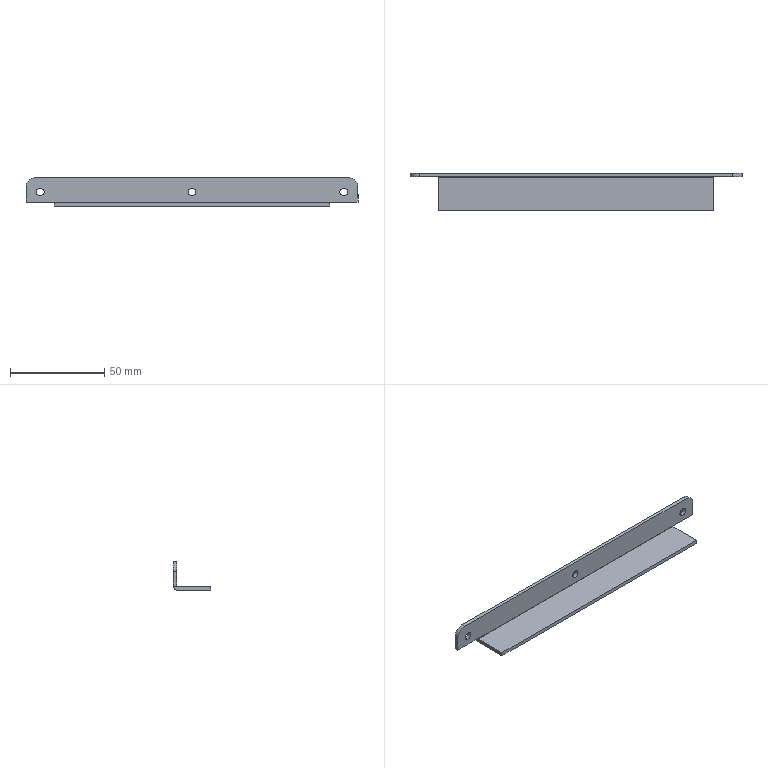Part | SolidWorks | features BaseBody 1 | 1 solid | 22 faces | box 176 x 20 x 15 mm | volume 10168 mm3 | plane 12 | cylinder 10 | commonest cylinder face diameters 4.2 x7 10 x2 0.2 x1
STEP:
#1=CARTESIAN_POINT('',(80.5,8.,3.4));
#2=VERTEX_POINT('',#1);
#3=CARTESIAN_POINT('',(80.5,8.,7.6));
#4=VERTEX_POINT('',#3);
#5=CARTESIAN_POINT('',(80.5,8.,5.5));
#6=DIRECTION('',(0.,1.,0.));
#7=DIRECTION('',(0.,0.,1.));
#8=AXIS2_PLACEMENT_3D('',#5,#6,#7);
#9=CIRCLE('',#8,2.1);
#10=EDGE_CURVE('',#2,#4,#9,.T.);
#11=ORIENTED_EDGE('',*,*,#10,.F.);
#12=CARTESIAN_POINT('',(80.5,10.,3.4));
#13=VERTEX_POINT('',#12);
#14=CARTESIAN_POINT('',(80.5,10.,3.4));
#15=DIRECTION('',(0.,1.,0.));
#16=VECTOR('',#15,1000.);
#17=LINE('',#14,#16);
#18=EDGE_CURVE('',#2,#13,#17,.T.);
#19=ORIENTED_EDGE('',*,*,#18,.T.);
#20=CARTESIAN_POINT('',(80.5,10.,7.6));
#21=VERTEX_POINT('',#20);
#22=CARTESIAN_POINT('',(80.5,10.,5.5));
#23=DIRECTION('',(0.,1.,0.));
#24=DIRECTION('',(0.,0.,1.));
#25=AXIS2_PLACEMENT_3D('',#22,#23,#24);
#26=CIRCLE('',#25,2.1);
#27=EDGE_CURVE('',#13,#21,#26,.T.);
#28=ORIENTED_EDGE('',*,*,#27,.T.);
#29=CARTESIAN_POINT('',(80.5,10.,7.6));
#30=DIRECTION('',(0.,1.,0.));
#31=VECTOR('',#30,1000.);
#32=LINE('',#29,#31);
#33=EDGE_CURVE('',#4,#21,#32,.T.);
#34=ORIENTED_EDGE('',*,*,#33,.F.);
#35=EDGE_LOOP('',(#11,#19,#28,#34));
#36=FACE_OUTER_BOUND('',#35,.T.);
#37=CARTESIAN_POINT('',(80.5,10.,5.5));
#38=DIRECTION('',(0.,1.,0.));
#39=DIRECTION('',(0.,0.,1.));
#40=AXIS2_PLACEMENT_3D('',#37,#38,#39);
#41=CYLINDRICAL_SURFACE('',#40,2.1);
#42=ADVANCED_FACE('',(#36),#41,.F.);
#43=CARTESIAN_POINT('',(0.,8.,3.4));
#44=VERTEX_POINT('',#43);
#45=CARTESIAN_POINT('',(0.,8.,7.6));
#46=VERTEX_POINT('',#45);
#47=CARTESIAN_POINT('',(0.,8.,5.5));
#48=DIRECTION('',(0.,1.,0.));
#49=DIRECTION('',(0.,0.,1.));
#50=AXIS2_PLACEMENT_3D('',#47,#48,#49);
#51=CIRCLE('',#50,2.1);
#52=EDGE_CURVE('',#44,#46,#51,.T.);
#53=ORIENTED_EDGE('',*,*,#52,.F.);
#54=CARTESIAN_POINT('',(0.,10.,3.4));
#55=VERTEX_POINT('',#54);
#56=CARTESIAN_POINT('',(0.,10.,3.4));
#57=DIRECTION('',(0.,1.,0.));
#58=VECTOR('',#57,1000.);
#59=LINE('',#56,#58);
#60=EDGE_CURVE('',#44,#55,#59,.T.);
#61=ORIENTED_EDGE('',*,*,#60,.T.);
#62=CARTESIAN_POINT('',(0.,10.,7.6));
#63=VERTEX_POINT('',#62);
#64=CARTESIAN_POINT('',(0.,10.,5.5));
#65=DIRECTION('',(0.,1.,0.));
#66=DIRECTION('',(0.,0.,1.));
#67=AXIS2_PLACEMENT_3D('',#64,#65,#66);
#68=CIRCLE('',#67,2.1);
#69=EDGE_CURVE('',#55,#63,#68,.T.);
#70=ORIENTED_EDGE('',*,*,#69,.T.);
#71=CARTESIAN_POINT('',(0.,10.,7.6));
#72=DIRECTION('',(0.,1.,0.));
#73=VECTOR('',#72,1000.);
#74=LINE('',#71,#73);
#75=EDGE_CURVE('',#46,#63,#74,.T.);
#76=ORIENTED_EDGE('',*,*,#75,.F.);
#77=EDGE_LOOP('',(#53,#61,#70,#76));
#78=FACE_OUTER_BOUND('',#77,.T.);
#79=CARTESIAN_POINT('',(0.,10.,5.5));
#80=DIRECTION('',(0.,1.,0.));
#81=DIRECTION('',(0.,0.,1.));
#82=AXIS2_PLACEMENT_3D('',#79,#80,#81);
#83=CYLINDRICAL_SURFACE('',#82,2.1);
#84=ADVANCED_FACE('',(#78),#83,.F.);
#85=CARTESIAN_POINT('',(-80.5,8.,3.4));
#86=VERTEX_POINT('',#85);
#87=CARTESIAN_POINT('',(-80.5,8.,7.6));
#88=VERTEX_POINT('',#87);
#89=CARTESIAN_POINT('',(-80.5,8.,5.5));
#90=DIRECTION('',(0.,1.,0.));
#91=DIRECTION('',(0.,0.,1.));
#92=AXIS2_PLACEMENT_3D('',#89,#90,#91);
#93=CIRCLE('',#92,2.1);
#94=EDGE_CURVE('',#86,#88,#93,.T.);
#95=ORIENTED_EDGE('',*,*,#94,.F.);
#96=CARTESIAN_POINT('',(-80.5,10.,3.4));
#97=VERTEX_POINT('',#96);
#98=CARTESIAN_POINT('',(-80.5,10.,3.4));
#99=DIRECTION('',(0.,1.,0.));
#100=VECTOR('',#99,1000.);
#101=LINE('',#98,#100);
#102=EDGE_CURVE('',#86,#97,#101,.T.);
#103=ORIENTED_EDGE('',*,*,#102,.T.);
#104=CARTESIAN_POINT('',(-80.5,10.,7.6));
#105=VERTEX_POINT('',#104);
#106=CARTESIAN_POINT('',(-80.5,10.,5.5));
#107=DIRECTION('',(0.,1.,0.));
#108=DIRECTION('',(0.,0.,1.));
#109=AXIS2_PLACEMENT_3D('',#106,#107,#108);
#110=CIRCLE('',#109,2.1);
#111=EDGE_CURVE('',#97,#105,#110,.T.);
#112=ORIENTED_EDGE('',*,*,#111,.T.);
#113=CARTESIAN_POINT('',(-80.5,10.,7.6));
#114=DIRECTION('',(0.,1.,0.));
#115=VECTOR('',#114,1000.);
#116=LINE('',#113,#115);
#117=EDGE_CURVE('',#88,#105,#116,.T.);
#118=ORIENTED_EDGE('',*,*,#117,.F.);
#119=EDGE_LOOP('',(#95,#103,#112,#118));
#120=FACE_OUTER_BOUND('',#119,.T.);
#121=CARTESIAN_POINT('',(-80.5,10.,5.5));
#122=DIRECTION('',(0.,1.,0.));
#123=DIRECTION('',(0.,0.,1.));
#124=AXIS2_PLACEMENT_3D('',#121,#122,#123);
#125=CYLINDRICAL_SURFACE('',#124,2.1);
#126=ADVANCED_FACE('',(#120),#125,.F.);
#127=CARTESIAN_POINT('',(73.,-10.,-2.));
#128=VERTEX_POINT('',#127);
#129=CARTESIAN_POINT('',(73.,7.9,-2.));
#130=VERTEX_POINT('',#129);
#131=CARTESIAN_POINT('',(73.,0.,-2.));
#132=DIRECTION('',(0.,1.,0.));
#133=VECTOR('',#132,1000.);
#134=LINE('',#131,#133);
#135=EDGE_CURVE('',#128,#130,#134,.T.);
#136=ORIENTED_EDGE('',*,*,#135,.F.);
#137=CARTESIAN_POINT('',(-73.,-10.,-2.));
#138=VERTEX_POINT('',#137);
#139=CARTESIAN_POINT('',(0.,-10.,-2.));
#140=DIRECTION('',(1.,0.,0.));
#141=VECTOR('',#140,1000.);
#142=LINE('',#139,#141);
#143=EDGE_CURVE('',#138,#128,#142,.T.);
#144=ORIENTED_EDGE('',*,*,#143,.F.);
#145=CARTESIAN_POINT('',(-73.,7.9,-2.));
#146=VERTEX_POINT('',#145);
#147=CARTESIAN_POINT('',(-73.,0.,-2.));
#148=DIRECTION('',(0.,-1.,0.));
#149=VECTOR('',#148,1000.);
#150=LINE('',#147,#149);
#151=EDGE_CURVE('',#146,#138,#150,.T.);
#152=ORIENTED_EDGE('',*,*,#151,.F.);
#153=CARTESIAN_POINT('',(0.,7.9,-2.));
#154=DIRECTION('',(-1.,0.,0.));
#155=VECTOR('',#154,1000.);
#156=LINE('',#153,#155);
#157=EDGE_CURVE('',#130,#146,#156,.T.);
#158=ORIENTED_EDGE('',*,*,#157,.F.);
#159=EDGE_LOOP('',(#136,#144,#152,#158));
#160=FACE_OUTER_BOUND('',#159,.T.);
#161=CARTESIAN_POINT('',(0.,0.,-2.));
#162=DIRECTION('',(0.,0.,1.));
#163=DIRECTION('',(1.,0.,0.));
#164=AXIS2_PLACEMENT_3D('',#161,#162,#163);
#165=PLANE('',#164);
#166=ADVANCED_FACE('',(#160),#165,.F.);
#167=CARTESIAN_POINT('',(-73.,10.,0.1));
#168=VERTEX_POINT('',#167);
#169=CARTESIAN_POINT('',(73.,10.,0.1));
#170=VERTEX_POINT('',#169);
#171=CARTESIAN_POINT('',(-73.,10.,0.1));
#172=DIRECTION('',(1.,0.,0.));
#173=VECTOR('',#172,1000.);
#174=LINE('',#171,#173);
#175=EDGE_CURVE('',#168,#170,#174,.T.);
#176=ORIENTED_EDGE('',*,*,#175,.T.);
#177=CARTESIAN_POINT('',(73.,7.9,0.1));
#178=DIRECTION('',(-1.,0.,0.));
#179=DIRECTION('',(0.,0.,1.));
#180=AXIS2_PLACEMENT_3D('',#177,#178,#179);
#181=CIRCLE('',#180,2.1);
#182=EDGE_CURVE('',#170,#130,#181,.T.);
#183=ORIENTED_EDGE('',*,*,#182,.T.);
#184=ORIENTED_EDGE('',*,*,#157,.T.);
#185=CARTESIAN_POINT('',(-73.,7.9,0.1));
#186=DIRECTION('',(1.,0.,0.));
#187=DIRECTION('',(0.,0.,1.));
#188=AXIS2_PLACEMENT_3D('',#185,#186,#187);
#189=CIRCLE('',#188,2.1);
#190=EDGE_CURVE('',#146,#168,#189,.T.);
#191=ORIENTED_EDGE('',*,*,#190,.T.);
#192=EDGE_LOOP('',(#176,#183,#184,#191));
#193=FACE_OUTER_BOUND('',#192,.T.);
#194=CARTESIAN_POINT('',(-73.,7.9,0.1));
#195=DIRECTION('',(-1.,0.,0.));
#196=DIRECTION('',(0.,0.,1.));
#197=AXIS2_PLACEMENT_3D('',#194,#195,#196);
#198=CYLINDRICAL_SURFACE('',#197,2.1);
#199=ADVANCED_FACE('',(#193),#198,.T.);
#200=CARTESIAN_POINT('',(73.,-10.,0.));
#201=VERTEX_POINT('',#200);
#202=CARTESIAN_POINT('',(73.,-10.,-2.));
#203=DIRECTION('',(0.,0.,-1.));
#204=VECTOR('',#203,1000.);
#205=LINE('',#202,#204);
#206=EDGE_CURVE('',#201,#128,#205,.T.);
#207=ORIENTED_EDGE('',*,*,#206,.T.);
#208=ORIENTED_EDGE('',*,*,#135,.T.);
#209=ORIENTED_EDGE('',*,*,#182,.F.);
#210=CARTESIAN_POINT('',(73.,8.,0.1));
#211=VERTEX_POINT('',#210);
#212=CARTESIAN_POINT('',(73.,7.9,0.1));
#213=DIRECTION('',(0.,-1.,0.));
#214=VECTOR('',#213,1000.);
#215=LINE('',#212,#214);
#216=EDGE_CURVE('',#170,#211,#215,.T.);
#217=ORIENTED_EDGE('',*,*,#216,.T.);
#218=CARTESIAN_POINT('',(73.,7.9,0.));
#219=VERTEX_POINT('',#218);
#220=CARTESIAN_POINT('',(73.,7.9,0.1));
#221=DIRECTION('',(-1.,0.,0.));
#222=DIRECTION('',(0.,0.,1.));
#223=AXIS2_PLACEMENT_3D('',#220,#221,#222);
#224=CIRCLE('',#223,0.1);
#225=EDGE_CURVE('',#211,#219,#224,.T.);
#226=ORIENTED_EDGE('',*,*,#225,.T.);
#227=CARTESIAN_POINT('',(73.,10.,0.));
#228=DIRECTION('',(0.,-1.,0.));
#229=VECTOR('',#228,1000.);
#230=LINE('',#227,#229);
#231=EDGE_CURVE('',#219,#201,#230,.T.);
#232=ORIENTED_EDGE('',*,*,#231,.T.);
#233=EDGE_LOOP('',(#207,#208,#209,#217,#226,#232));
#234=FACE_OUTER_BOUND('',#233,.T.);
#235=CARTESIAN_POINT('',(73.,10.,-2.));
#236=DIRECTION('',(1.,0.,0.));
#237=DIRECTION('',(0.,0.,-1.));
#238=AXIS2_PLACEMENT_3D('',#235,#236,#237);
#239=PLANE('',#238);
#240=ADVANCED_FACE('',(#234),#239,.T.);
#241=ORIENTED_EDGE('',*,*,#143,.T.);
#242=ORIENTED_EDGE('',*,*,#206,.F.);
#243=CARTESIAN_POINT('',(-73.,-10.,0.));
#244=VERTEX_POINT('',#243);
#245=CARTESIAN_POINT('',(-73.,-10.,0.));
#246=DIRECTION('',(-1.,0.,0.));
#247=VECTOR('',#246,1000.);
#248=LINE('',#245,#247);
#249=EDGE_CURVE('',#201,#244,#248,.T.);
#250=ORIENTED_EDGE('',*,*,#249,.T.);
#251=CARTESIAN_POINT('',(-73.,-10.,-2.));
#252=DIRECTION('',(0.,0.,-1.));
#253=VECTOR('',#252,1000.);
#254=LINE('',#251,#253);
#255=EDGE_CURVE('',#244,#138,#254,.T.);
#256=ORIENTED_EDGE('',*,*,#255,.T.);
#257=EDGE_LOOP('',(#241,#242,#250,#256));
#258=FACE_OUTER_BOUND('',#257,.T.);
#259=CARTESIAN_POINT('',(-73.,-10.,-2.));
#260=DIRECTION('',(0.,-1.,0.));
#261=DIRECTION('',(0.,0.,-1.));
#262=AXIS2_PLACEMENT_3D('',#259,#260,#261);
#263=PLANE('',#262);
#264=ADVANCED_FACE('',(#258),#263,.T.);
#265=ORIENTED_EDGE('',*,*,#151,.T.);
#266=ORIENTED_EDGE('',*,*,#255,.F.);
#267=CARTESIAN_POINT('',(-73.,7.9,0.));
#268=VERTEX_POINT('',#267);
#269=CARTESIAN_POINT('',(-73.,10.,0.));
#270=DIRECTION('',(0.,1.,0.));
#271=VECTOR('',#270,1000.);
#272=LINE('',#269,#271);
#273=EDGE_CURVE('',#244,#268,#272,.T.);
#274=ORIENTED_EDGE('',*,*,#273,.T.);
#275=CARTESIAN_POINT('',(-73.,8.,0.1));
#276=VERTEX_POINT('',#275);
#277=CARTESIAN_POINT('',(-73.,7.9,0.1));
#278=DIRECTION('',(1.,0.,0.));
#279=DIRECTION('',(0.,0.,1.));
#280=AXIS2_PLACEMENT_3D('',#277,#278,#279);
#281=CIRCLE('',#280,0.1);
#282=EDGE_CURVE('',#268,#276,#281,.T.);
#283=ORIENTED_EDGE('',*,*,#282,.T.);
#284=CARTESIAN_POINT('',(-73.,7.9,0.1));
#285=DIRECTION('',(0.,-1.,0.));
#286=VECTOR('',#285,1000.);
#287=LINE('',#284,#286);
#288=EDGE_CURVE('',#168,#276,#287,.T.);
#289=ORIENTED_EDGE('',*,*,#288,.F.);
#290=ORIENTED_EDGE('',*,*,#190,.F.);
#291=EDGE_LOOP('',(#265,#266,#274,#283,#289,#290));
#292=FACE_OUTER_BOUND('',#291,.T.);
#293=CARTESIAN_POINT('',(-73.,10.,-2.));
#294=DIRECTION('',(-1.,0.,0.));
#295=DIRECTION('',(0.,0.,1.));
#296=AXIS2_PLACEMENT_3D('',#293,#294,#295);
#297=PLANE('',#296);
#298=ADVANCED_FACE('',(#292),#297,.T.);
#299=CARTESIAN_POINT('',(88.,10.,8.));
#300=VERTEX_POINT('',#299);
#301=CARTESIAN_POINT('',(83.,10.,13.));
#302=VERTEX_POINT('',#301);
#303=CARTESIAN_POINT('',(83.,10.,8.));
#304=DIRECTION('',(0.,-1.,0.));
#305=DIRECTION('',(0.,0.,1.));
#306=AXIS2_PLACEMENT_3D('',#303,#304,#305);
#307=CIRCLE('',#306,5.);
#308=EDGE_CURVE('',#300,#302,#307,.T.);
#309=ORIENTED_EDGE('',*,*,#308,.F.);
#310=CARTESIAN_POINT('',(88.,10.,0.1));
#311=VERTEX_POINT('',#310);
#312=CARTESIAN_POINT('',(88.,10.,0.));
#313=DIRECTION('',(0.,0.,1.));
#314=VECTOR('',#313,1000.);
#315=LINE('',#312,#314);
#316=EDGE_CURVE('',#311,#300,#315,.T.);
#317=ORIENTED_EDGE('',*,*,#316,.F.);
#318=CARTESIAN_POINT('',(0.,10.,0.1));
#319=DIRECTION('',(1.,0.,0.));
#320=VECTOR('',#319,1000.);
#321=LINE('',#318,#320);
#322=EDGE_CURVE('',#170,#311,#321,.T.);
#323=ORIENTED_EDGE('',*,*,#322,.F.);
#324=ORIENTED_EDGE('',*,*,#175,.F.);
#325=CARTESIAN_POINT('',(-88.,10.,0.1));
#326=VERTEX_POINT('',#325);
#327=CARTESIAN_POINT('',(0.,10.,0.1));
#328=DIRECTION('',(1.,0.,0.));
#329=VECTOR('',#328,1000.);
#330=LINE('',#327,#329);
#331=EDGE_CURVE('',#326,#168,#330,.T.);
#332=ORIENTED_EDGE('',*,*,#331,.F.);
#333=CARTESIAN_POINT('',(-88.,10.,8.));
#334=VERTEX_POINT('',#333);
#335=CARTESIAN_POINT('',(-88.,10.,0.));
#336=DIRECTION('',(0.,0.,-1.));
#337=VECTOR('',#336,1000.);
#338=LINE('',#335,#337);
#339=EDGE_CURVE('',#334,#326,#338,.T.);
#340=ORIENTED_EDGE('',*,*,#339,.F.);
#341=CARTESIAN_POINT('',(-83.,10.,13.));
#342=VERTEX_POINT('',#341);
#343=CARTESIAN_POINT('',(-83.,10.,8.));
#344=DIRECTION('',(0.,-1.,0.));
#345=DIRECTION('',(0.,0.,-1.));
#346=AXIS2_PLACEMENT_3D('',#343,#344,#345);
#347=CIRCLE('',#346,5.);
#348=EDGE_CURVE('',#342,#334,#347,.T.);
#349=ORIENTED_EDGE('',*,*,#348,.F.);
#350=CARTESIAN_POINT('',(0.,10.,13.));
#351=DIRECTION('',(-1.,0.,0.));
#352=VECTOR('',#351,1000.);
#353=LINE('',#350,#352);
#354=EDGE_CURVE('',#302,#342,#353,.T.);
#355=ORIENTED_EDGE('',*,*,#354,.F.);
#356=EDGE_LOOP('',(#309,#317,#323,#324,#332,#340,#349,#355));
#357=FACE_OUTER_BOUND('',#356,.T.);
#358=CARTESIAN_POINT('',(80.5,10.,5.5));
#359=DIRECTION('',(0.,1.,0.));
#360=DIRECTION('',(0.,0.,1.));
#361=AXIS2_PLACEMENT_3D('',#358,#359,#360);
#362=CIRCLE('',#361,2.1);
#363=EDGE_CURVE('',#21,#13,#362,.T.);
#364=ORIENTED_EDGE('',*,*,#363,.F.);
#365=ORIENTED_EDGE('',*,*,#27,.F.);
#366=EDGE_LOOP('',(#364,#365));
#367=FACE_BOUND('',#366,.T.);
#368=CARTESIAN_POINT('',(0.,10.,5.5));
#369=DIRECTION('',(0.,1.,0.));
#370=DIRECTION('',(0.,0.,1.));
#371=AXIS2_PLACEMENT_3D('',#368,#369,#370);
#372=CIRCLE('',#371,2.1);
#373=EDGE_CURVE('',#63,#55,#372,.T.);
#374=ORIENTED_EDGE('',*,*,#373,.F.);
#375=ORIENTED_EDGE('',*,*,#69,.F.);
#376=EDGE_LOOP('',(#374,#375));
#377=FACE_BOUND('',#376,.T.);
#378=CARTESIAN_POINT('',(-80.5,10.,5.5));
#379=DIRECTION('',(0.,1.,0.));
#380=DIRECTION('',(0.,0.,1.));
#381=AXIS2_PLACEMENT_3D('',#378,#379,#380);
#382=CIRCLE('',#381,2.1);
#383=EDGE_CURVE('',#105,#97,#382,.T.);
#384=ORIENTED_EDGE('',*,*,#383,.F.);
#385=ORIENTED_EDGE('',*,*,#111,.F.);
#386=EDGE_LOOP('',(#384,#385));
#387=FACE_BOUND('',#386,.T.);
#388=CARTESIAN_POINT('',(0.,10.,0.));
#389=DIRECTION('',(0.,-1.,0.));
#390=DIRECTION('',(0.,0.,-1.));
#391=AXIS2_PLACEMENT_3D('',#388,#389,#390);
#392=PLANE('',#391);
#393=ADVANCED_FACE('',(#357,#367,#377,#387),#392,.F.);
#394=ORIENTED_EDGE('',*,*,#273,.F.);
#395=ORIENTED_EDGE('',*,*,#249,.F.);
#396=ORIENTED_EDGE('',*,*,#231,.F.);
#397=CARTESIAN_POINT('',(0.,7.9,0.));
#398=DIRECTION('',(-1.,0.,0.));
#399=VECTOR('',#398,1000.);
#400=LINE('',#397,#399);
#401=EDGE_CURVE('',#219,#268,#400,.T.);
#402=ORIENTED_EDGE('',*,*,#401,.T.);
#403=EDGE_LOOP('',(#394,#395,#396,#402));
#404=FACE_OUTER_BOUND('',#403,.T.);
#405=CARTESIAN_POINT('',(0.,0.,0.));
#406=DIRECTION('',(0.,0.,1.));
#407=DIRECTION('',(1.,0.,0.));
#408=AXIS2_PLACEMENT_3D('',#405,#406,#407);
#409=PLANE('',#408);
#410=ADVANCED_FACE('',(#404),#409,.T.);
#411=ORIENTED_EDGE('',*,*,#322,.T.);
#412=CARTESIAN_POINT('',(88.,8.,0.1));
#413=VERTEX_POINT('',#412);
#414=CARTESIAN_POINT('',(88.,8.,0.1));
#415=DIRECTION('',(0.,1.,0.));
#416=VECTOR('',#415,1000.);
#417=LINE('',#414,#416);
#418=EDGE_CURVE('',#413,#311,#417,.T.);
#419=ORIENTED_EDGE('',*,*,#418,.F.);
#420=CARTESIAN_POINT('',(88.,8.,0.1));
#421=DIRECTION('',(1.,0.,0.));
#422=VECTOR('',#421,1000.);
#423=LINE('',#420,#422);
#424=EDGE_CURVE('',#211,#413,#423,.T.);
#425=ORIENTED_EDGE('',*,*,#424,.F.);
#426=ORIENTED_EDGE('',*,*,#216,.F.);
#427=EDGE_LOOP('',(#411,#419,#425,#426));
#428=FACE_OUTER_BOUND('',#427,.T.);
#429=CARTESIAN_POINT('',(88.,8.,0.1));
#430=DIRECTION('',(0.,0.,1.));
#431=DIRECTION('',(0.,-1.,0.));
#432=AXIS2_PLACEMENT_3D('',#429,#430,#431);
#433=PLANE('',#432);
#434=ADVANCED_FACE('',(#428),#433,.F.);
#435=CARTESIAN_POINT('',(83.,8.,13.));
#436=VERTEX_POINT('',#435);
#437=CARTESIAN_POINT('',(83.,10.,13.));
#438=DIRECTION('',(0.,-1.,0.));
#439=VECTOR('',#438,1000.);
#440=LINE('',#437,#439);
#441=EDGE_CURVE('',#302,#436,#440,.T.);
#442=ORIENTED_EDGE('',*,*,#441,.F.);
#443=ORIENTED_EDGE('',*,*,#354,.T.);
#444=CARTESIAN_POINT('',(-83.,8.,13.));
#445=VERTEX_POINT('',#444);
#446=CARTESIAN_POINT('',(-83.,10.,13.));
#447=DIRECTION('',(0.,1.,0.));
#448=VECTOR('',#447,1000.);
#449=LINE('',#446,#448);
#450=EDGE_CURVE('',#445,#342,#449,.T.);
#451=ORIENTED_EDGE('',*,*,#450,.F.);
#452=CARTESIAN_POINT('',(73.,8.,13.));
#453=DIRECTION('',(-1.,0.,0.));
#454=VECTOR('',#453,1000.);
#455=LINE('',#452,#454);
#456=EDGE_CURVE('',#436,#445,#455,.T.);
#457=ORIENTED_EDGE('',*,*,#456,.F.);
#458=EDGE_LOOP('',(#442,#443,#451,#457));
#459=FACE_OUTER_BOUND('',#458,.T.);
#460=CARTESIAN_POINT('',(73.,10.,13.));
#461=DIRECTION('',(0.,0.,-1.));
#462=DIRECTION('',(0.,1.,0.));
#463=AXIS2_PLACEMENT_3D('',#460,#461,#462);
#464=PLANE('',#463);
#465=ADVANCED_FACE('',(#459),#464,.F.);
#466=CARTESIAN_POINT('',(88.,8.,8.));
#467=VERTEX_POINT('',#466);
#468=CARTESIAN_POINT('',(83.,8.,8.));
#469=DIRECTION('',(0.,1.,0.));
#470=DIRECTION('',(0.,0.,1.));
#471=AXIS2_PLACEMENT_3D('',#468,#469,#470);
#472=CIRCLE('',#471,5.);
#473=EDGE_CURVE('',#436,#467,#472,.T.);
#474=ORIENTED_EDGE('',*,*,#473,.T.);
#475=CARTESIAN_POINT('',(88.,0.,8.));
#476=DIRECTION('',(0.,1.,0.));
#477=VECTOR('',#476,1000.);
#478=LINE('',#475,#477);
#479=EDGE_CURVE('',#467,#300,#478,.T.);
#480=ORIENTED_EDGE('',*,*,#479,.T.);
#481=ORIENTED_EDGE('',*,*,#308,.T.);
#482=ORIENTED_EDGE('',*,*,#441,.T.);
#483=EDGE_LOOP('',(#474,#480,#481,#482));
#484=FACE_OUTER_BOUND('',#483,.T.);
#485=CARTESIAN_POINT('',(83.,0.,8.));
#486=DIRECTION('',(0.,1.,0.));
#487=DIRECTION('',(0.,0.,1.));
#488=AXIS2_PLACEMENT_3D('',#485,#486,#487);
#489=CYLINDRICAL_SURFACE('',#488,5.);
#490=ADVANCED_FACE('',(#484),#489,.T.);
#491=CARTESIAN_POINT('',(88.,8.,0.));
#492=DIRECTION('',(0.,0.,-1.));
#493=VECTOR('',#492,1000.);
#494=LINE('',#491,#493);
#495=EDGE_CURVE('',#467,#413,#494,.T.);
#496=ORIENTED_EDGE('',*,*,#495,.T.);
#497=ORIENTED_EDGE('',*,*,#418,.T.);
#498=ORIENTED_EDGE('',*,*,#316,.T.);
#499=ORIENTED_EDGE('',*,*,#479,.F.);
#500=EDGE_LOOP('',(#496,#497,#498,#499));
#501=FACE_OUTER_BOUND('',#500,.T.);
#502=CARTESIAN_POINT('',(88.,0.,0.));
#503=DIRECTION('',(1.,0.,0.));
#504=DIRECTION('',(0.,0.,-1.));
#505=AXIS2_PLACEMENT_3D('',#502,#503,#504);
#506=PLANE('',#505);
#507=ADVANCED_FACE('',(#501),#506,.T.);
#508=CARTESIAN_POINT('',(-88.,8.,0.1));
#509=VERTEX_POINT('',#508);
#510=CARTESIAN_POINT('',(-88.,8.,0.1));
#511=DIRECTION('',(1.,0.,0.));
#512=VECTOR('',#511,1000.);
#513=LINE('',#510,#512);
#514=EDGE_CURVE('',#509,#276,#513,.T.);
#515=ORIENTED_EDGE('',*,*,#514,.F.);
#516=CARTESIAN_POINT('',(-88.,10.,0.1));
#517=DIRECTION('',(0.,-1.,0.));
#518=VECTOR('',#517,1000.);
#519=LINE('',#516,#518);
#520=EDGE_CURVE('',#326,#509,#519,.T.);
#521=ORIENTED_EDGE('',*,*,#520,.F.);
#522=ORIENTED_EDGE('',*,*,#331,.T.);
#523=ORIENTED_EDGE('',*,*,#288,.T.);
#524=EDGE_LOOP('',(#515,#521,#522,#523));
#525=FACE_OUTER_BOUND('',#524,.T.);
#526=CARTESIAN_POINT('',(-88.,10.,0.1));
#527=DIRECTION('',(0.,0.,1.));
#528=DIRECTION('',(0.,-1.,0.));
#529=AXIS2_PLACEMENT_3D('',#526,#527,#528);
#530=PLANE('',#529);
#531=ADVANCED_FACE('',(#525),#530,.F.);
#532=ORIENTED_EDGE('',*,*,#339,.T.);
#533=ORIENTED_EDGE('',*,*,#520,.T.);
#534=CARTESIAN_POINT('',(-88.,8.,8.));
#535=VERTEX_POINT('',#534);
#536=CARTESIAN_POINT('',(-88.,8.,0.));
#537=DIRECTION('',(0.,0.,1.));
#538=VECTOR('',#537,1000.);
#539=LINE('',#536,#538);
#540=EDGE_CURVE('',#509,#535,#539,.T.);
#541=ORIENTED_EDGE('',*,*,#540,.T.);
#542=CARTESIAN_POINT('',(-88.,0.,8.));
#543=DIRECTION('',(0.,1.,0.));
#544=VECTOR('',#543,1000.);
#545=LINE('',#542,#544);
#546=EDGE_CURVE('',#535,#334,#545,.T.);
#547=ORIENTED_EDGE('',*,*,#546,.T.);
#548=EDGE_LOOP('',(#532,#533,#541,#547));
#549=FACE_OUTER_BOUND('',#548,.T.);
#550=CARTESIAN_POINT('',(-88.,0.,0.));
#551=DIRECTION('',(-1.,0.,0.));
#552=DIRECTION('',(0.,0.,1.));
#553=AXIS2_PLACEMENT_3D('',#550,#551,#552);
#554=PLANE('',#553);
#555=ADVANCED_FACE('',(#549),#554,.T.);
#556=ORIENTED_EDGE('',*,*,#348,.T.);
#557=ORIENTED_EDGE('',*,*,#546,.F.);
#558=CARTESIAN_POINT('',(-83.,8.,8.));
#559=DIRECTION('',(0.,1.,0.));
#560=DIRECTION('',(0.,0.,-1.));
#561=AXIS2_PLACEMENT_3D('',#558,#559,#560);
#562=CIRCLE('',#561,5.);
#563=EDGE_CURVE('',#535,#445,#562,.T.);
#564=ORIENTED_EDGE('',*,*,#563,.T.);
#565=ORIENTED_EDGE('',*,*,#450,.T.);
#566=EDGE_LOOP('',(#556,#557,#564,#565));
#567=FACE_OUTER_BOUND('',#566,.T.);
#568=CARTESIAN_POINT('',(-83.,0.,8.));
#569=DIRECTION('',(0.,-1.,0.));
#570=DIRECTION('',(0.,0.,-1.));
#571=AXIS2_PLACEMENT_3D('',#568,#569,#570);
#572=CYLINDRICAL_SURFACE('',#571,5.);
#573=ADVANCED_FACE('',(#567),#572,.T.);
#574=ORIENTED_EDGE('',*,*,#18,.F.);
#575=CARTESIAN_POINT('',(80.5,8.,5.5));
#576=DIRECTION('',(0.,1.,0.));
#577=DIRECTION('',(0.,0.,1.));
#578=AXIS2_PLACEMENT_3D('',#575,#576,#577);
#579=CIRCLE('',#578,2.1);
#580=EDGE_CURVE('',#4,#2,#579,.T.);
#581=ORIENTED_EDGE('',*,*,#580,.F.);
#582=ORIENTED_EDGE('',*,*,#33,.T.);
#583=ORIENTED_EDGE('',*,*,#363,.T.);
#584=EDGE_LOOP('',(#574,#581,#582,#583));
#585=FACE_OUTER_BOUND('',#584,.T.);
#586=CARTESIAN_POINT('',(80.5,10.,5.5));
#587=DIRECTION('',(0.,1.,0.));
#588=DIRECTION('',(0.,0.,1.));
#589=AXIS2_PLACEMENT_3D('',#586,#587,#588);
#590=CYLINDRICAL_SURFACE('',#589,2.1);
#591=ADVANCED_FACE('',(#585),#590,.F.);
#592=ORIENTED_EDGE('',*,*,#60,.F.);
#593=CARTESIAN_POINT('',(0.,8.,5.5));
#594=DIRECTION('',(0.,1.,0.));
#595=DIRECTION('',(0.,0.,1.));
#596=AXIS2_PLACEMENT_3D('',#593,#594,#595);
#597=CIRCLE('',#596,2.1);
#598=EDGE_CURVE('',#46,#44,#597,.T.);
#599=ORIENTED_EDGE('',*,*,#598,.F.);
#600=ORIENTED_EDGE('',*,*,#75,.T.);
#601=ORIENTED_EDGE('',*,*,#373,.T.);
#602=EDGE_LOOP('',(#592,#599,#600,#601));
#603=FACE_OUTER_BOUND('',#602,.T.);
#604=CARTESIAN_POINT('',(0.,10.,5.5));
#605=DIRECTION('',(0.,1.,0.));
#606=DIRECTION('',(0.,0.,1.));
#607=AXIS2_PLACEMENT_3D('',#604,#605,#606);
#608=CYLINDRICAL_SURFACE('',#607,2.1);
#609=ADVANCED_FACE('',(#603),#608,.F.);
#610=ORIENTED_EDGE('',*,*,#102,.F.);
#611=CARTESIAN_POINT('',(-80.5,8.,5.5));
#612=DIRECTION('',(0.,1.,0.));
#613=DIRECTION('',(0.,0.,1.));
#614=AXIS2_PLACEMENT_3D('',#611,#612,#613);
#615=CIRCLE('',#614,2.1);
#616=EDGE_CURVE('',#88,#86,#615,.T.);
#617=ORIENTED_EDGE('',*,*,#616,.F.);
#618=ORIENTED_EDGE('',*,*,#117,.T.);
#619=ORIENTED_EDGE('',*,*,#383,.T.);
#620=EDGE_LOOP('',(#610,#617,#618,#619));
#621=FACE_OUTER_BOUND('',#620,.T.);
#622=CARTESIAN_POINT('',(-80.5,10.,5.5));
#623=DIRECTION('',(0.,1.,0.));
#624=DIRECTION('',(0.,0.,1.));
#625=AXIS2_PLACEMENT_3D('',#622,#623,#624);
#626=CYLINDRICAL_SURFACE('',#625,2.1);
#627=ADVANCED_FACE('',(#621),#626,.F.);
#628=ORIENTED_EDGE('',*,*,#225,.F.);
#629=CARTESIAN_POINT('',(-73.,8.,0.1));
#630=DIRECTION('',(1.,0.,0.));
#631=VECTOR('',#630,1000.);
#632=LINE('',#629,#631);
#633=EDGE_CURVE('',#276,#211,#632,.T.);
#634=ORIENTED_EDGE('',*,*,#633,.F.);
#635=ORIENTED_EDGE('',*,*,#282,.F.);
#636=ORIENTED_EDGE('',*,*,#401,.F.);
#637=EDGE_LOOP('',(#628,#634,#635,#636));
#638=FACE_OUTER_BOUND('',#637,.T.);
#639=CARTESIAN_POINT('',(-73.,7.9,0.1));
#640=DIRECTION('',(-1.,0.,0.));
#641=DIRECTION('',(0.,0.,1.));
#642=AXIS2_PLACEMENT_3D('',#639,#640,#641);
#643=CYLINDRICAL_SURFACE('',#642,0.1);
#644=ADVANCED_FACE('',(#638),#643,.F.);
#645=ORIENTED_EDGE('',*,*,#633,.T.);
#646=ORIENTED_EDGE('',*,*,#424,.T.);
#647=ORIENTED_EDGE('',*,*,#495,.F.);
#648=ORIENTED_EDGE('',*,*,#473,.F.);
#649=ORIENTED_EDGE('',*,*,#456,.T.);
#650=ORIENTED_EDGE('',*,*,#563,.F.);
#651=ORIENTED_EDGE('',*,*,#540,.F.);
#652=ORIENTED_EDGE('',*,*,#514,.T.);
#653=EDGE_LOOP('',(#645,#646,#647,#648,#649,#650,#651,#652));
#654=FACE_OUTER_BOUND('',#653,.T.);
#655=ORIENTED_EDGE('',*,*,#580,.T.);
#656=ORIENTED_EDGE('',*,*,#10,.T.);
#657=EDGE_LOOP('',(#655,#656));
#658=FACE_BOUND('',#657,.T.);
#659=ORIENTED_EDGE('',*,*,#598,.T.);
#660=ORIENTED_EDGE('',*,*,#52,.T.);
#661=EDGE_LOOP('',(#659,#660));
#662=FACE_BOUND('',#661,.T.);
#663=ORIENTED_EDGE('',*,*,#616,.T.);
#664=ORIENTED_EDGE('',*,*,#94,.T.);
#665=EDGE_LOOP('',(#663,#664));
#666=FACE_BOUND('',#665,.T.);
#667=CARTESIAN_POINT('',(0.,8.,0.));
#668=DIRECTION('',(0.,-1.,0.));
#669=DIRECTION('',(0.,0.,-1.));
#670=AXIS2_PLACEMENT_3D('',#667,#668,#669);
#671=PLANE('',#670);
#672=ADVANCED_FACE('',(#654,#658,#662,#666),#671,.T.);
#673=CLOSED_SHELL('',(#42,#84,#126,#166,#199,#240,#264,#298,#393,#410,#434,#465,#490,#507,#531,#555,#573,#591,#609,#627,#644,#672));
#674=MANIFOLD_SOLID_BREP('',#673);
#675=CARTESIAN_POINT('',(0.,0.,0.));
#676=DIRECTION('',(0.,0.,1.));
#677=DIRECTION('',(1.,0.,0.));
#678=AXIS2_PLACEMENT_3D('',#675,#676,#677);
#679=(LENGTH_UNIT()NAMED_UNIT(*)SI_UNIT(.MILLI.,.METRE.));
#680=UNCERTAINTY_MEASURE_WITH_UNIT(LENGTH_MEASURE(0.00001),#679,'','');
#681=(NAMED_UNIT(*)PLANE_ANGLE_UNIT()SI_UNIT($,.RADIAN.));
#682=(NAMED_UNIT(*)SI_UNIT($,.STERADIAN.)SOLID_ANGLE_UNIT());
#683=(GEOMETRIC_REPRESENTATION_CONTEXT(3)GLOBAL_UNCERTAINTY_ASSIGNED_CONTEXT((#680))GLOBAL_UNIT_ASSIGNED_CONTEXT((#679,#681,#682))REPRESENTATION_CONTEXT('',''));
#684=ADVANCED_BREP_SHAPE_REPRESENTATION('',(#674,#678),#683);